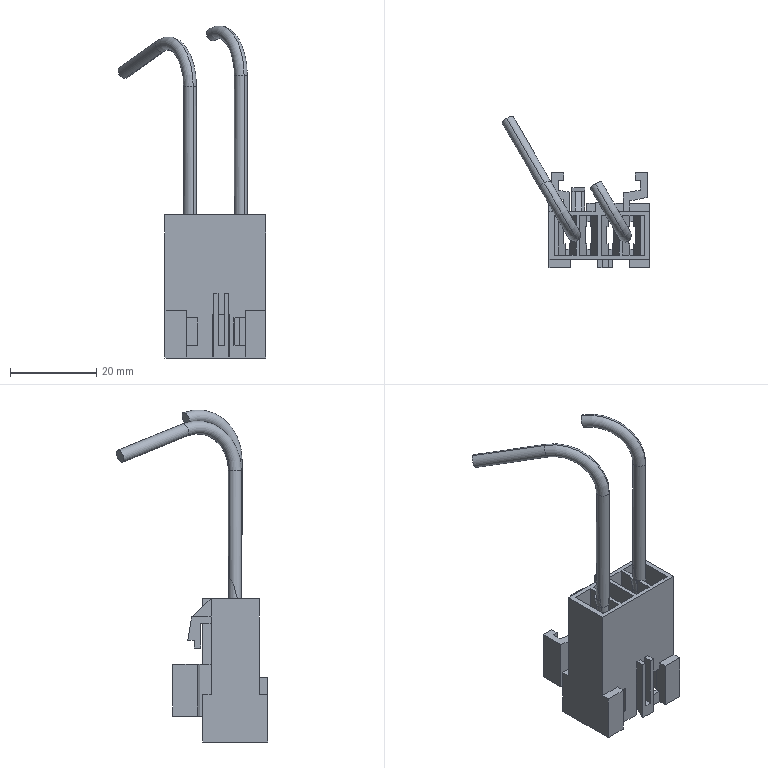Part | STEP file | MSBR-16_1_5_4_1_1 | 1 solid | 238 faces | box 34.276 x 35.044 x 77.065 mm | volume 5583 mm3 | plane 212 | cylinder 17 | torus 9 | commonest cylinder face diameters 3 x13 92 x2 96 x2